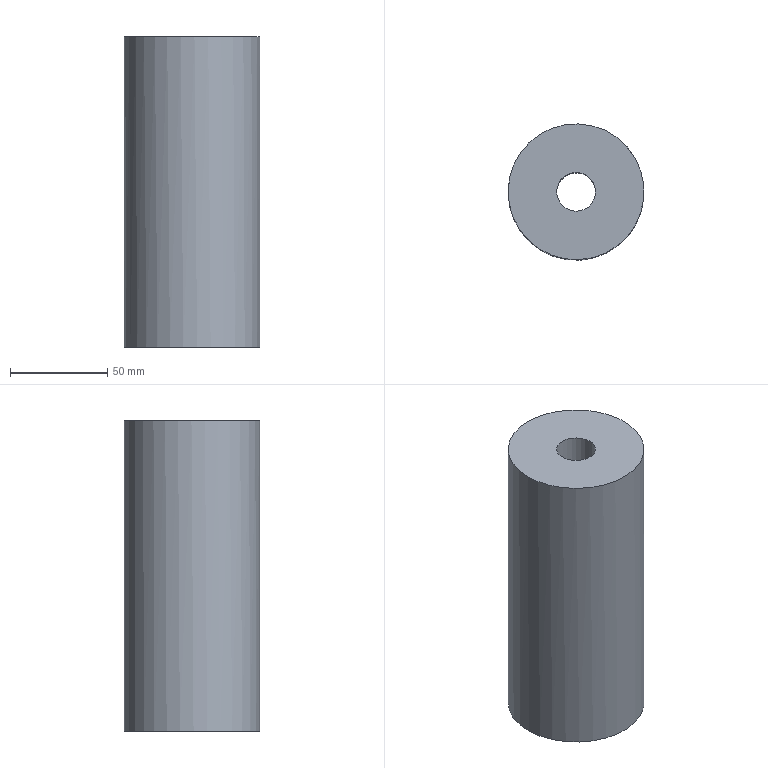Part | NX | features solid 2 | 1 solid | 4 faces | box 70 x 70 x 160 mm | volume 565487 mm3 | plane 2 | cylinder 2 | commonest cylinder face diameters 20 x1 70 x1
STEP:
#1=CARTESIAN_POINT('',(-1544.749,815.251,81.6));
#2=VERTEX_POINT('',#1);
#3=CARTESIAN_POINT('',(-1520.,840.,81.6));
#4=DIRECTION('',(0.,0.,1.));
#5=DIRECTION('',(-0.7071,-0.7071,0.));
#6=AXIS2_PLACEMENT_3D('',#3,#4,#5);
#7=CIRCLE('',#6,35.);
#8=EDGE_CURVE('',#2,#2,#7,.F.);
#9=ORIENTED_EDGE('',*,*,#8,.F.);
#10=EDGE_LOOP('',(#9));
#11=FACE_BOUND('',#10,.T.);
#12=CARTESIAN_POINT('',(-1527.071,832.929,81.6));
#13=VERTEX_POINT('',#12);
#14=CARTESIAN_POINT('',(-1520.,840.,81.6));
#15=DIRECTION('',(0.,0.,1.));
#16=DIRECTION('',(-0.7071,-0.7071,0.));
#17=AXIS2_PLACEMENT_3D('',#14,#15,#16);
#18=CIRCLE('',#17,10.);
#19=EDGE_CURVE('',#13,#13,#18,.F.);
#20=ORIENTED_EDGE('',*,*,#19,.T.);
#21=EDGE_LOOP('',(#20));
#22=FACE_BOUND('',#21,.T.);
#23=CARTESIAN_POINT('',(-1520.,840.,81.6));
#24=DIRECTION('',(0.,0.,-1.));
#25=DIRECTION('',(0.1736,-0.9848,0.));
#26=AXIS2_PLACEMENT_3D('',#23,#24,#25);
#27=PLANE('',#26);
#28=ADVANCED_FACE('',(#11,#22),#27,.F.);
#29=CARTESIAN_POINT('',(-1526.078,874.468,-78.4));
#30=VERTEX_POINT('',#29);
#31=CARTESIAN_POINT('',(-1520.,840.,-78.4));
#32=DIRECTION('',(0.,0.,-1.));
#33=DIRECTION('',(-0.1736,0.9848,0.));
#34=AXIS2_PLACEMENT_3D('',#31,#32,#33);
#35=CIRCLE('',#34,35.);
#36=EDGE_CURVE('',#30,#30,#35,.T.);
#37=ORIENTED_EDGE('',*,*,#36,.T.);
#38=EDGE_LOOP('',(#37));
#39=FACE_BOUND('',#38,.T.);
#40=CARTESIAN_POINT('',(-1521.736,849.848,-78.4));
#41=VERTEX_POINT('',#40);
#42=CARTESIAN_POINT('',(-1520.,840.,-78.4));
#43=DIRECTION('',(0.,0.,-1.));
#44=DIRECTION('',(-0.1736,0.9848,0.));
#45=AXIS2_PLACEMENT_3D('',#42,#43,#44);
#46=CIRCLE('',#45,10.);
#47=EDGE_CURVE('',#41,#41,#46,.T.);
#48=ORIENTED_EDGE('',*,*,#47,.F.);
#49=EDGE_LOOP('',(#48));
#50=FACE_BOUND('',#49,.T.);
#51=CARTESIAN_POINT('',(-1520.,840.,-78.4));
#52=DIRECTION('',(0.,0.,-1.));
#53=DIRECTION('',(0.1736,-0.9848,0.));
#54=AXIS2_PLACEMENT_3D('',#51,#52,#53);
#55=PLANE('',#54);
#56=ADVANCED_FACE('',(#39,#50),#55,.T.);
#57=ORIENTED_EDGE('',*,*,#8,.T.);
#58=EDGE_LOOP('',(#57));
#59=FACE_BOUND('',#58,.T.);
#60=ORIENTED_EDGE('',*,*,#36,.F.);
#61=EDGE_LOOP('',(#60));
#62=FACE_BOUND('',#61,.T.);
#63=CARTESIAN_POINT('',(-1520.,840.,-78.4));
#64=DIRECTION('',(0.,0.,1.));
#65=DIRECTION('',(-0.1736,0.9848,0.));
#66=AXIS2_PLACEMENT_3D('',#63,#64,#65);
#67=CYLINDRICAL_SURFACE('',#66,35.);
#68=ADVANCED_FACE('',(#59,#62),#67,.T.);
#69=ORIENTED_EDGE('',*,*,#19,.F.);
#70=EDGE_LOOP('',(#69));
#71=FACE_BOUND('',#70,.T.);
#72=ORIENTED_EDGE('',*,*,#47,.T.);
#73=EDGE_LOOP('',(#72));
#74=FACE_BOUND('',#73,.T.);
#75=CARTESIAN_POINT('',(-1520.,840.,-78.4));
#76=DIRECTION('',(0.,0.,1.));
#77=DIRECTION('',(-0.1736,0.9848,0.));
#78=AXIS2_PLACEMENT_3D('',#75,#76,#77);
#79=CYLINDRICAL_SURFACE('',#78,10.);
#80=ADVANCED_FACE('',(#71,#74),#79,.F.);
#81=CLOSED_SHELL('',(#28,#56,#68,#80));
#82=MANIFOLD_SOLID_BREP('',#81);
#83=(LENGTH_UNIT()NAMED_UNIT(*)SI_UNIT(.MILLI.,.METRE.));
#84=UNCERTAINTY_MEASURE_WITH_UNIT(LENGTH_MEASURE(0.00001),#83,'','');
#85=(NAMED_UNIT(*)PLANE_ANGLE_UNIT()SI_UNIT($,.RADIAN.));
#86=(NAMED_UNIT(*)SI_UNIT($,.STERADIAN.)SOLID_ANGLE_UNIT());
#87=(GEOMETRIC_REPRESENTATION_CONTEXT(3)GLOBAL_UNCERTAINTY_ASSIGNED_CONTEXT((#84))GLOBAL_UNIT_ASSIGNED_CONTEXT((#83,#85,#86))REPRESENTATION_CONTEXT('',''));
#88=ADVANCED_BREP_SHAPE_REPRESENTATION('',(#82),#87);